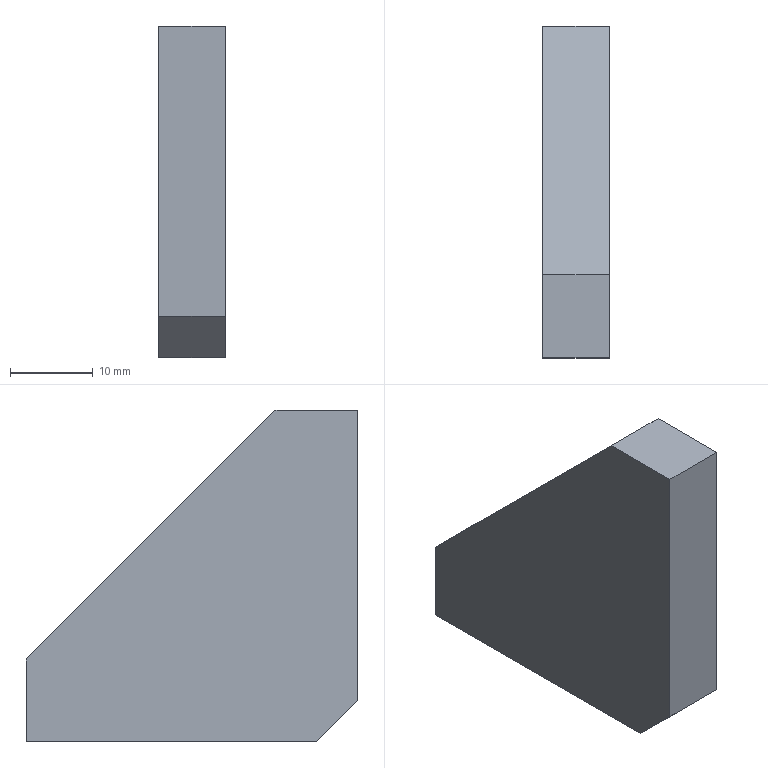Part | SolidWorks | features FlatPattern 1, SMBaseFlange 1, SheetMetal 1 | 1 solid | 8 faces | box 8 x 40 x 40 mm | volume 9100 mm3 | plane 8
STEP:
#1=CARTESIAN_POINT('',(0.,40.,0.));
#2=VERTEX_POINT('',#1);
#3=CARTESIAN_POINT('',(0.,40.,10.));
#4=VERTEX_POINT('',#3);
#5=CARTESIAN_POINT('',(0.,40.,0.));
#6=DIRECTION('',(0.,0.,1.));
#7=VECTOR('',#6,1000.);
#8=LINE('',#5,#7);
#9=EDGE_CURVE('',#2,#4,#8,.T.);
#10=ORIENTED_EDGE('',*,*,#9,.F.);
#11=CARTESIAN_POINT('',(-8.,40.,0.));
#12=VERTEX_POINT('',#11);
#13=CARTESIAN_POINT('',(-8.,40.,0.));
#14=DIRECTION('',(1.,0.,0.));
#15=VECTOR('',#14,1000.);
#16=LINE('',#13,#15);
#17=EDGE_CURVE('',#12,#2,#16,.T.);
#18=ORIENTED_EDGE('',*,*,#17,.F.);
#19=CARTESIAN_POINT('',(-8.,40.,10.));
#20=VERTEX_POINT('',#19);
#21=CARTESIAN_POINT('',(-8.,40.,0.));
#22=DIRECTION('',(0.,0.,1.));
#23=VECTOR('',#22,1000.);
#24=LINE('',#21,#23);
#25=EDGE_CURVE('',#12,#20,#24,.T.);
#26=ORIENTED_EDGE('',*,*,#25,.T.);
#27=CARTESIAN_POINT('',(-8.,40.,10.));
#28=DIRECTION('',(1.,0.,0.));
#29=VECTOR('',#28,1000.);
#30=LINE('',#27,#29);
#31=EDGE_CURVE('',#20,#4,#30,.T.);
#32=ORIENTED_EDGE('',*,*,#31,.T.);
#33=EDGE_LOOP('',(#10,#18,#26,#32));
#34=FACE_OUTER_BOUND('',#33,.T.);
#35=CARTESIAN_POINT('',(-8.,40.,0.));
#36=DIRECTION('',(0.,1.,0.));
#37=DIRECTION('',(0.,0.,1.));
#38=AXIS2_PLACEMENT_3D('',#35,#36,#37);
#39=PLANE('',#38);
#40=ADVANCED_FACE('',(#34),#39,.T.);
#41=CARTESIAN_POINT('',(0.,5.,0.));
#42=VERTEX_POINT('',#41);
#43=CARTESIAN_POINT('',(0.,5.,0.));
#44=DIRECTION('',(0.,1.,0.));
#45=VECTOR('',#44,1000.);
#46=LINE('',#43,#45);
#47=EDGE_CURVE('',#42,#2,#46,.T.);
#48=ORIENTED_EDGE('',*,*,#47,.F.);
#49=CARTESIAN_POINT('',(-8.,5.,0.));
#50=VERTEX_POINT('',#49);
#51=CARTESIAN_POINT('',(-8.,5.,0.));
#52=DIRECTION('',(1.,0.,0.));
#53=VECTOR('',#52,1000.);
#54=LINE('',#51,#53);
#55=EDGE_CURVE('',#50,#42,#54,.T.);
#56=ORIENTED_EDGE('',*,*,#55,.F.);
#57=CARTESIAN_POINT('',(-8.,5.,0.));
#58=DIRECTION('',(0.,1.,0.));
#59=VECTOR('',#58,1000.);
#60=LINE('',#57,#59);
#61=EDGE_CURVE('',#50,#12,#60,.T.);
#62=ORIENTED_EDGE('',*,*,#61,.T.);
#63=ORIENTED_EDGE('',*,*,#17,.T.);
#64=EDGE_LOOP('',(#48,#56,#62,#63));
#65=FACE_OUTER_BOUND('',#64,.T.);
#66=CARTESIAN_POINT('',(-8.,5.,0.));
#67=DIRECTION('',(0.,0.,-1.));
#68=DIRECTION('',(-1.,0.,0.));
#69=AXIS2_PLACEMENT_3D('',#66,#67,#68);
#70=PLANE('',#69);
#71=ADVANCED_FACE('',(#65),#70,.T.);
#72=CARTESIAN_POINT('',(0.,0.,5.));
#73=VERTEX_POINT('',#72);
#74=CARTESIAN_POINT('',(0.,0.,5.));
#75=DIRECTION('',(0.,0.7071,-0.7071));
#76=VECTOR('',#75,1000.);
#77=LINE('',#74,#76);
#78=EDGE_CURVE('',#73,#42,#77,.T.);
#79=ORIENTED_EDGE('',*,*,#78,.F.);
#80=CARTESIAN_POINT('',(-8.,0.,5.));
#81=VERTEX_POINT('',#80);
#82=CARTESIAN_POINT('',(-8.,0.,5.));
#83=DIRECTION('',(1.,0.,0.));
#84=VECTOR('',#83,1000.);
#85=LINE('',#82,#84);
#86=EDGE_CURVE('',#81,#73,#85,.T.);
#87=ORIENTED_EDGE('',*,*,#86,.F.);
#88=CARTESIAN_POINT('',(-8.,0.,5.));
#89=DIRECTION('',(0.,0.7071,-0.7071));
#90=VECTOR('',#89,1000.);
#91=LINE('',#88,#90);
#92=EDGE_CURVE('',#81,#50,#91,.T.);
#93=ORIENTED_EDGE('',*,*,#92,.T.);
#94=ORIENTED_EDGE('',*,*,#55,.T.);
#95=EDGE_LOOP('',(#79,#87,#93,#94));
#96=FACE_OUTER_BOUND('',#95,.T.);
#97=CARTESIAN_POINT('',(-8.,0.,5.));
#98=DIRECTION('',(0.,-0.7071,-0.7071));
#99=DIRECTION('',(0.,0.7071,-0.7071));
#100=AXIS2_PLACEMENT_3D('',#97,#98,#99);
#101=PLANE('',#100);
#102=ADVANCED_FACE('',(#96),#101,.T.);
#103=CARTESIAN_POINT('',(0.,0.,40.));
#104=VERTEX_POINT('',#103);
#105=CARTESIAN_POINT('',(0.,0.,40.));
#106=DIRECTION('',(0.,0.,-1.));
#107=VECTOR('',#106,1000.);
#108=LINE('',#105,#107);
#109=EDGE_CURVE('',#104,#73,#108,.T.);
#110=ORIENTED_EDGE('',*,*,#109,.F.);
#111=CARTESIAN_POINT('',(-8.,0.,40.));
#112=VERTEX_POINT('',#111);
#113=CARTESIAN_POINT('',(-8.,0.,40.));
#114=DIRECTION('',(1.,0.,0.));
#115=VECTOR('',#114,1000.);
#116=LINE('',#113,#115);
#117=EDGE_CURVE('',#112,#104,#116,.T.);
#118=ORIENTED_EDGE('',*,*,#117,.F.);
#119=CARTESIAN_POINT('',(-8.,0.,40.));
#120=DIRECTION('',(0.,0.,-1.));
#121=VECTOR('',#120,1000.);
#122=LINE('',#119,#121);
#123=EDGE_CURVE('',#112,#81,#122,.T.);
#124=ORIENTED_EDGE('',*,*,#123,.T.);
#125=ORIENTED_EDGE('',*,*,#86,.T.);
#126=EDGE_LOOP('',(#110,#118,#124,#125));
#127=FACE_OUTER_BOUND('',#126,.T.);
#128=CARTESIAN_POINT('',(-8.,0.,40.));
#129=DIRECTION('',(0.,-1.,0.));
#130=DIRECTION('',(0.,0.,-1.));
#131=AXIS2_PLACEMENT_3D('',#128,#129,#130);
#132=PLANE('',#131);
#133=ADVANCED_FACE('',(#127),#132,.T.);
#134=CARTESIAN_POINT('',(0.,10.,40.));
#135=VERTEX_POINT('',#134);
#136=CARTESIAN_POINT('',(0.,10.,40.));
#137=DIRECTION('',(0.,-1.,0.));
#138=VECTOR('',#137,1000.);
#139=LINE('',#136,#138);
#140=EDGE_CURVE('',#135,#104,#139,.T.);
#141=ORIENTED_EDGE('',*,*,#140,.F.);
#142=CARTESIAN_POINT('',(-8.,10.,40.));
#143=VERTEX_POINT('',#142);
#144=CARTESIAN_POINT('',(-8.,10.,40.));
#145=DIRECTION('',(1.,0.,0.));
#146=VECTOR('',#145,1000.);
#147=LINE('',#144,#146);
#148=EDGE_CURVE('',#143,#135,#147,.T.);
#149=ORIENTED_EDGE('',*,*,#148,.F.);
#150=CARTESIAN_POINT('',(-8.,10.,40.));
#151=DIRECTION('',(0.,-1.,0.));
#152=VECTOR('',#151,1000.);
#153=LINE('',#150,#152);
#154=EDGE_CURVE('',#143,#112,#153,.T.);
#155=ORIENTED_EDGE('',*,*,#154,.T.);
#156=ORIENTED_EDGE('',*,*,#117,.T.);
#157=EDGE_LOOP('',(#141,#149,#155,#156));
#158=FACE_OUTER_BOUND('',#157,.T.);
#159=CARTESIAN_POINT('',(-8.,10.,40.));
#160=DIRECTION('',(0.,0.,1.));
#161=DIRECTION('',(1.,0.,0.));
#162=AXIS2_PLACEMENT_3D('',#159,#160,#161);
#163=PLANE('',#162);
#164=ADVANCED_FACE('',(#158),#163,.T.);
#165=CARTESIAN_POINT('',(0.,40.,10.));
#166=DIRECTION('',(0.,-0.7071,0.7071));
#167=VECTOR('',#166,1000.);
#168=LINE('',#165,#167);
#169=EDGE_CURVE('',#4,#135,#168,.T.);
#170=ORIENTED_EDGE('',*,*,#169,.F.);
#171=ORIENTED_EDGE('',*,*,#31,.F.);
#172=CARTESIAN_POINT('',(-8.,40.,10.));
#173=DIRECTION('',(0.,-0.7071,0.7071));
#174=VECTOR('',#173,1000.);
#175=LINE('',#172,#174);
#176=EDGE_CURVE('',#20,#143,#175,.T.);
#177=ORIENTED_EDGE('',*,*,#176,.T.);
#178=ORIENTED_EDGE('',*,*,#148,.T.);
#179=EDGE_LOOP('',(#170,#171,#177,#178));
#180=FACE_OUTER_BOUND('',#179,.T.);
#181=CARTESIAN_POINT('',(-8.,40.,10.));
#182=DIRECTION('',(0.,0.7071,0.7071));
#183=DIRECTION('',(0.,-0.7071,0.7071));
#184=AXIS2_PLACEMENT_3D('',#181,#182,#183);
#185=PLANE('',#184);
#186=ADVANCED_FACE('',(#180),#185,.T.);
#187=ORIENTED_EDGE('',*,*,#25,.F.);
#188=ORIENTED_EDGE('',*,*,#61,.F.);
#189=ORIENTED_EDGE('',*,*,#92,.F.);
#190=ORIENTED_EDGE('',*,*,#123,.F.);
#191=ORIENTED_EDGE('',*,*,#154,.F.);
#192=ORIENTED_EDGE('',*,*,#176,.F.);
#193=EDGE_LOOP('',(#187,#188,#189,#190,#191,#192));
#194=FACE_OUTER_BOUND('',#193,.T.);
#195=CARTESIAN_POINT('',(-8.,0.,0.));
#196=DIRECTION('',(1.,0.,0.));
#197=DIRECTION('',(0.,0.,-1.));
#198=AXIS2_PLACEMENT_3D('',#195,#196,#197);
#199=PLANE('',#198);
#200=ADVANCED_FACE('',(#194),#199,.F.);
#201=ORIENTED_EDGE('',*,*,#9,.T.);
#202=ORIENTED_EDGE('',*,*,#169,.T.);
#203=ORIENTED_EDGE('',*,*,#140,.T.);
#204=ORIENTED_EDGE('',*,*,#109,.T.);
#205=ORIENTED_EDGE('',*,*,#78,.T.);
#206=ORIENTED_EDGE('',*,*,#47,.T.);
#207=EDGE_LOOP('',(#201,#202,#203,#204,#205,#206));
#208=FACE_OUTER_BOUND('',#207,.T.);
#209=CARTESIAN_POINT('',(0.,0.,0.));
#210=DIRECTION('',(1.,0.,0.));
#211=DIRECTION('',(0.,0.,-1.));
#212=AXIS2_PLACEMENT_3D('',#209,#210,#211);
#213=PLANE('',#212);
#214=ADVANCED_FACE('',(#208),#213,.T.);
#215=CLOSED_SHELL('',(#40,#71,#102,#133,#164,#186,#200,#214));
#216=MANIFOLD_SOLID_BREP('',#215);
#217=CARTESIAN_POINT('',(0.,0.,0.));
#218=DIRECTION('',(0.,0.,1.));
#219=DIRECTION('',(1.,0.,0.));
#220=AXIS2_PLACEMENT_3D('',#217,#218,#219);
#221=(LENGTH_UNIT()NAMED_UNIT(*)SI_UNIT(.MILLI.,.METRE.));
#222=UNCERTAINTY_MEASURE_WITH_UNIT(LENGTH_MEASURE(0.00001),#221,'','');
#223=(NAMED_UNIT(*)PLANE_ANGLE_UNIT()SI_UNIT($,.RADIAN.));
#224=(NAMED_UNIT(*)SI_UNIT($,.STERADIAN.)SOLID_ANGLE_UNIT());
#225=(GEOMETRIC_REPRESENTATION_CONTEXT(3)GLOBAL_UNCERTAINTY_ASSIGNED_CONTEXT((#222))GLOBAL_UNIT_ASSIGNED_CONTEXT((#221,#223,#224))REPRESENTATION_CONTEXT('',''));
#226=ADVANCED_BREP_SHAPE_REPRESENTATION('',(#216,#220),#225);